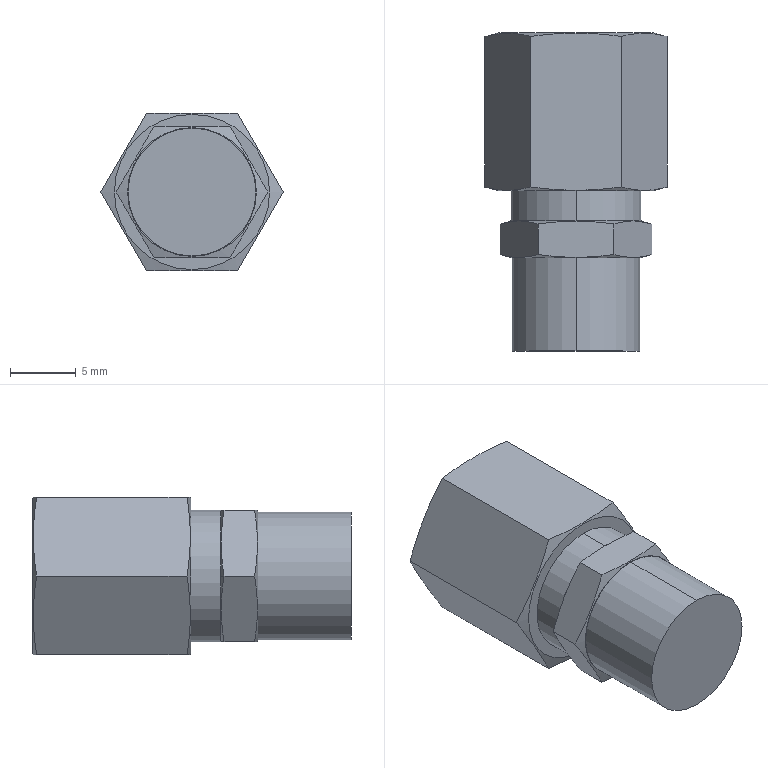Part | STEP file | H06-01S | 1 solid | 32 faces | box 13.856 x 24.2 x 12 mm | volume 1991 mm3 | plane 18 | cone 8 | cylinder 6 | commonest cylinder face diameters 6 x2 9.728 x2 10 x2
STEP:
#1=CARTESIAN_POINT('',(0.,5.1,-3.));
#2=VERTEX_POINT('',#1);
#3=CARTESIAN_POINT('',(0.,5.1,3.));
#4=VERTEX_POINT('',#3);
#5=CARTESIAN_POINT('',(0.,5.1,0.));
#6=DIRECTION('',(0.,1.,0.));
#7=DIRECTION('',(0.,0.,1.));
#8=AXIS2_PLACEMENT_3D('',#5,#6,#7);
#9=CIRCLE('',#8,3.);
#10=EDGE_CURVE('',#2,#4,#9,.T.);
#11=ORIENTED_EDGE('',*,*,#10,.F.);
#12=CARTESIAN_POINT('',(0.,21.1,-3.));
#13=VERTEX_POINT('',#12);
#14=CARTESIAN_POINT('',(0.,5.1,-3.));
#15=DIRECTION('',(0.,1.,0.));
#16=VECTOR('',#15,1000.);
#17=LINE('',#14,#16);
#18=EDGE_CURVE('',#2,#13,#17,.T.);
#19=ORIENTED_EDGE('',*,*,#18,.T.);
#20=CARTESIAN_POINT('',(0.,21.1,3.));
#21=VERTEX_POINT('',#20);
#22=CARTESIAN_POINT('',(0.,21.1,0.));
#23=DIRECTION('',(0.,-1.,0.));
#24=DIRECTION('',(0.,0.,1.));
#25=AXIS2_PLACEMENT_3D('',#22,#23,#24);
#26=CIRCLE('',#25,3.);
#27=EDGE_CURVE('',#21,#13,#26,.T.);
#28=ORIENTED_EDGE('',*,*,#27,.F.);
#29=CARTESIAN_POINT('',(0.,5.1,3.));
#30=DIRECTION('',(0.,1.,0.));
#31=VECTOR('',#30,1000.);
#32=LINE('',#29,#31);
#33=EDGE_CURVE('',#4,#21,#32,.T.);
#34=ORIENTED_EDGE('',*,*,#33,.F.);
#35=EDGE_LOOP('',(#11,#19,#28,#34));
#36=FACE_OUTER_BOUND('',#35,.T.);
#37=CARTESIAN_POINT('',(0.,5.1,0.));
#38=DIRECTION('',(0.,1.,0.));
#39=DIRECTION('',(0.,0.,1.));
#40=AXIS2_PLACEMENT_3D('',#37,#38,#39);
#41=CYLINDRICAL_SURFACE('',#40,3.);
#42=ADVANCED_FACE('',(#36),#41,.F.);
#43=CARTESIAN_POINT('',(0.,21.1,-5.9));
#44=VERTEX_POINT('',#43);
#45=CARTESIAN_POINT('',(0.,21.1,5.9));
#46=VERTEX_POINT('',#45);
#47=CARTESIAN_POINT('',(0.,21.1,0.));
#48=DIRECTION('',(0.,-1.,0.));
#49=DIRECTION('',(0.,0.,-1.));
#50=AXIS2_PLACEMENT_3D('',#47,#48,#49);
#51=CIRCLE('',#50,5.9);
#52=EDGE_CURVE('',#44,#46,#51,.T.);
#53=ORIENTED_EDGE('',*,*,#52,.T.);
#54=CARTESIAN_POINT('',(0.,21.073,6.));
#55=VERTEX_POINT('',#54);
#56=CARTESIAN_POINT('',(0.,20.823,6.934));
#57=DIRECTION('',(0.,-0.2588,0.9659));
#58=VECTOR('',#57,1000.);
#59=LINE('',#56,#58);
#60=EDGE_CURVE('',#46,#55,#59,.T.);
#61=ORIENTED_EDGE('',*,*,#60,.T.);
#62=CARTESIAN_POINT('',(3.464,20.824,6.));
#63=VERTEX_POINT('',#62);
#64=CARTESIAN_POINT('',(0.,21.073,6.));
#65=CARTESIAN_POINT('',(1.155,21.073,6.));
#66=CARTESIAN_POINT('',(2.309,20.979,6.));
#67=CARTESIAN_POINT('',(3.464,20.824,6.));
#68=B_SPLINE_CURVE_WITH_KNOTS('',3,(#64,#65,#66,#67),.UNSPECIFIED.,.F.,.F.,(4,4),(0.003464,0.006928),.UNSPECIFIED.);
#69=EDGE_CURVE('',#55,#63,#68,.T.);
#70=ORIENTED_EDGE('',*,*,#69,.T.);
#71=CARTESIAN_POINT('',(6.928,20.824,0.000000051));
#72=VERTEX_POINT('',#71);
#73=CARTESIAN_POINT('',(3.464,20.824,6.));
#74=CARTESIAN_POINT('',(4.041,20.979,5.));
#75=CARTESIAN_POINT('',(5.196,21.167,3.));
#76=CARTESIAN_POINT('',(6.351,20.979,1.));
#77=CARTESIAN_POINT('',(6.928,20.824,0.000000051));
#78=B_SPLINE_CURVE_WITH_KNOTS('',3,(#73,#74,#75,#76,#77),.UNSPECIFIED.,.F.,.F.,(4,1,4),(0.,0.003464,0.006928),.UNSPECIFIED.);
#79=EDGE_CURVE('',#63,#72,#78,.T.);
#80=ORIENTED_EDGE('',*,*,#79,.T.);
#81=CARTESIAN_POINT('',(3.464,20.824,-6.));
#82=VERTEX_POINT('',#81);
#83=CARTESIAN_POINT('',(6.928,20.824,0.000000051));
#84=CARTESIAN_POINT('',(6.351,20.979,-1.));
#85=CARTESIAN_POINT('',(5.196,21.167,-3.));
#86=CARTESIAN_POINT('',(4.041,20.979,-5.));
#87=CARTESIAN_POINT('',(3.464,20.824,-6.));
#88=B_SPLINE_CURVE_WITH_KNOTS('',3,(#83,#84,#85,#86,#87),.UNSPECIFIED.,.F.,.F.,(4,1,4),(0.,0.003464,0.006928),.UNSPECIFIED.);
#89=EDGE_CURVE('',#72,#82,#88,.T.);
#90=ORIENTED_EDGE('',*,*,#89,.T.);
#91=CARTESIAN_POINT('',(0.,21.073,-6.));
#92=VERTEX_POINT('',#91);
#93=CARTESIAN_POINT('',(3.464,20.824,-6.));
#94=CARTESIAN_POINT('',(2.309,20.979,-6.));
#95=CARTESIAN_POINT('',(1.155,21.073,-6.));
#96=CARTESIAN_POINT('',(0.,21.073,-6.));
#97=B_SPLINE_CURVE_WITH_KNOTS('',3,(#93,#94,#95,#96),.UNSPECIFIED.,.F.,.F.,(4,4),(0.,0.003464),.UNSPECIFIED.);
#98=EDGE_CURVE('',#82,#92,#97,.T.);
#99=ORIENTED_EDGE('',*,*,#98,.T.);
#100=CARTESIAN_POINT('',(0.,20.823,-6.934));
#101=DIRECTION('',(0.,-0.2588,-0.9659));
#102=VECTOR('',#101,1000.);
#103=LINE('',#100,#102);
#104=EDGE_CURVE('',#44,#92,#103,.T.);
#105=ORIENTED_EDGE('',*,*,#104,.F.);
#106=EDGE_LOOP('',(#53,#61,#70,#80,#90,#99,#105));
#107=FACE_OUTER_BOUND('',#106,.T.);
#108=CARTESIAN_POINT('',(0.,20.823,0.));
#109=DIRECTION('',(0.,-1.,0.));
#110=DIRECTION('',(0.,0.,-1.));
#111=AXIS2_PLACEMENT_3D('',#108,#109,#110);
#112=CONICAL_SURFACE('',#111,6.934,1.309);
#113=ADVANCED_FACE('',(#107),#112,.T.);
#114=CARTESIAN_POINT('',(0.,9.1,5.9));
#115=VERTEX_POINT('',#114);
#116=CARTESIAN_POINT('',(0.,9.1,-5.9));
#117=VERTEX_POINT('',#116);
#118=CARTESIAN_POINT('',(0.,9.1,0.));
#119=DIRECTION('',(0.,1.,0.));
#120=DIRECTION('',(0.,0.,1.));
#121=AXIS2_PLACEMENT_3D('',#118,#119,#120);
#122=CIRCLE('',#121,5.9);
#123=EDGE_CURVE('',#115,#117,#122,.T.);
#124=ORIENTED_EDGE('',*,*,#123,.T.);
#125=CARTESIAN_POINT('',(0.,9.127,-6.));
#126=VERTEX_POINT('',#125);
#127=CARTESIAN_POINT('',(0.,9.377,-6.934));
#128=DIRECTION('',(0.,0.2588,-0.9659));
#129=VECTOR('',#128,1000.);
#130=LINE('',#127,#129);
#131=EDGE_CURVE('',#117,#126,#130,.T.);
#132=ORIENTED_EDGE('',*,*,#131,.T.);
#133=CARTESIAN_POINT('',(3.464,9.376,-6.));
#134=VERTEX_POINT('',#133);
#135=CARTESIAN_POINT('',(3.464,9.376,-6.));
#136=CARTESIAN_POINT('',(2.309,9.221,-6.));
#137=CARTESIAN_POINT('',(1.155,9.127,-6.));
#138=CARTESIAN_POINT('',(0.,9.127,-6.));
#139=B_SPLINE_CURVE_WITH_KNOTS('',3,(#135,#136,#137,#138),.UNSPECIFIED.,.F.,.F.,(4,4),(0.,0.003464),.UNSPECIFIED.);
#140=EDGE_CURVE('',#134,#126,#139,.T.);
#141=ORIENTED_EDGE('',*,*,#140,.F.);
#142=CARTESIAN_POINT('',(6.928,9.376,0.));
#143=VERTEX_POINT('',#142);
#144=CARTESIAN_POINT('',(6.928,9.376,0.));
#145=CARTESIAN_POINT('',(6.351,9.221,-1.));
#146=CARTESIAN_POINT('',(5.196,9.033,-3.));
#147=CARTESIAN_POINT('',(4.041,9.221,-5.));
#148=CARTESIAN_POINT('',(3.464,9.376,-6.));
#149=B_SPLINE_CURVE_WITH_KNOTS('',3,(#144,#145,#146,#147,#148),.UNSPECIFIED.,.F.,.F.,(4,1,4),(0.,0.003464,0.006928),.UNSPECIFIED.);
#150=EDGE_CURVE('',#143,#134,#149,.T.);
#151=ORIENTED_EDGE('',*,*,#150,.F.);
#152=CARTESIAN_POINT('',(3.464,9.376,6.));
#153=VERTEX_POINT('',#152);
#154=CARTESIAN_POINT('',(3.464,9.376,6.));
#155=CARTESIAN_POINT('',(4.041,9.221,5.));
#156=CARTESIAN_POINT('',(5.196,9.033,3.));
#157=CARTESIAN_POINT('',(6.351,9.221,1.));
#158=CARTESIAN_POINT('',(6.928,9.376,0.));
#159=B_SPLINE_CURVE_WITH_KNOTS('',3,(#154,#155,#156,#157,#158),.UNSPECIFIED.,.F.,.F.,(4,1,4),(0.,0.003464,0.006928),.UNSPECIFIED.);
#160=EDGE_CURVE('',#153,#143,#159,.T.);
#161=ORIENTED_EDGE('',*,*,#160,.F.);
#162=CARTESIAN_POINT('',(0.,9.127,6.));
#163=VERTEX_POINT('',#162);
#164=CARTESIAN_POINT('',(0.,9.127,6.));
#165=CARTESIAN_POINT('',(1.155,9.127,6.));
#166=CARTESIAN_POINT('',(2.309,9.221,6.));
#167=CARTESIAN_POINT('',(3.464,9.376,6.));
#168=B_SPLINE_CURVE_WITH_KNOTS('',3,(#164,#165,#166,#167),.UNSPECIFIED.,.F.,.F.,(4,4),(0.003464,0.006928),.UNSPECIFIED.);
#169=EDGE_CURVE('',#163,#153,#168,.T.);
#170=ORIENTED_EDGE('',*,*,#169,.F.);
#171=CARTESIAN_POINT('',(0.,9.377,6.934));
#172=DIRECTION('',(0.,0.2588,0.9659));
#173=VECTOR('',#172,1000.);
#174=LINE('',#171,#173);
#175=EDGE_CURVE('',#115,#163,#174,.T.);
#176=ORIENTED_EDGE('',*,*,#175,.F.);
#177=EDGE_LOOP('',(#124,#132,#141,#151,#161,#170,#176));
#178=FACE_OUTER_BOUND('',#177,.T.);
#179=CARTESIAN_POINT('',(0.,9.377,0.));
#180=DIRECTION('',(0.,1.,0.));
#181=DIRECTION('',(0.,0.,1.));
#182=AXIS2_PLACEMENT_3D('',#179,#180,#181);
#183=CONICAL_SURFACE('',#182,6.934,1.309);
#184=ADVANCED_FACE('',(#178),#183,.T.);
#185=CARTESIAN_POINT('',(0.,9.1,-5.));
#186=VERTEX_POINT('',#185);
#187=CARTESIAN_POINT('',(0.,9.1,5.));
#188=VERTEX_POINT('',#187);
#189=CARTESIAN_POINT('',(0.,9.1,0.));
#190=DIRECTION('',(0.,-1.,0.));
#191=DIRECTION('',(0.,0.,-1.));
#192=AXIS2_PLACEMENT_3D('',#189,#190,#191);
#193=CIRCLE('',#192,5.);
#194=EDGE_CURVE('',#186,#188,#193,.T.);
#195=ORIENTED_EDGE('',*,*,#194,.T.);
#196=CARTESIAN_POINT('',(0.,6.8,5.));
#197=VERTEX_POINT('',#196);
#198=CARTESIAN_POINT('',(0.,21.1,5.));
#199=DIRECTION('',(0.,-1.,0.));
#200=VECTOR('',#199,1000.);
#201=LINE('',#198,#200);
#202=EDGE_CURVE('',#188,#197,#201,.T.);
#203=ORIENTED_EDGE('',*,*,#202,.T.);
#204=CARTESIAN_POINT('',(0.,6.8,-5.));
#205=VERTEX_POINT('',#204);
#206=CARTESIAN_POINT('',(0.,6.8,0.));
#207=DIRECTION('',(0.,1.,0.));
#208=DIRECTION('',(0.,0.,-1.));
#209=AXIS2_PLACEMENT_3D('',#206,#207,#208);
#210=CIRCLE('',#209,5.);
#211=EDGE_CURVE('',#197,#205,#210,.T.);
#212=ORIENTED_EDGE('',*,*,#211,.T.);
#213=CARTESIAN_POINT('',(0.,21.1,-5.));
#214=DIRECTION('',(0.,-1.,0.));
#215=VECTOR('',#214,1000.);
#216=LINE('',#213,#215);
#217=EDGE_CURVE('',#186,#205,#216,.T.);
#218=ORIENTED_EDGE('',*,*,#217,.F.);
#219=EDGE_LOOP('',(#195,#203,#212,#218));
#220=FACE_OUTER_BOUND('',#219,.T.);
#221=CARTESIAN_POINT('',(0.,21.1,0.));
#222=DIRECTION('',(0.,-1.,0.));
#223=DIRECTION('',(0.,0.,-1.));
#224=AXIS2_PLACEMENT_3D('',#221,#222,#223);
#225=CYLINDRICAL_SURFACE('',#224,5.);
#226=ADVANCED_FACE('',(#220),#225,.T.);
#227=CARTESIAN_POINT('',(4.9,6.8,0.));
#228=VERTEX_POINT('',#227);
#229=CARTESIAN_POINT('',(-4.9,6.8,0.));
#230=VERTEX_POINT('',#229);
#231=CARTESIAN_POINT('',(0.,6.8,0.));
#232=DIRECTION('',(0.,-1.,0.));
#233=DIRECTION('',(1.,0.,0.));
#234=AXIS2_PLACEMENT_3D('',#231,#232,#233);
#235=CIRCLE('',#234,4.9);
#236=EDGE_CURVE('',#228,#230,#235,.T.);
#237=ORIENTED_EDGE('',*,*,#236,.T.);
#238=CARTESIAN_POINT('',(-5.774,6.566,-0.000000051));
#239=VERTEX_POINT('',#238);
#240=CARTESIAN_POINT('',(-5.779,6.565,0.));
#241=DIRECTION('',(-0.9659,-0.2588,0.));
#242=VECTOR('',#241,1000.);
#243=LINE('',#240,#242);
#244=EDGE_CURVE('',#230,#239,#243,.T.);
#245=ORIENTED_EDGE('',*,*,#244,.T.);
#246=CARTESIAN_POINT('',(-2.887,6.566,5.));
#247=VERTEX_POINT('',#246);
#248=CARTESIAN_POINT('',(-5.774,6.566,-0.000000051));
#249=CARTESIAN_POINT('',(-5.292,6.695,0.8333));
#250=CARTESIAN_POINT('',(-4.33,6.852,2.5));
#251=CARTESIAN_POINT('',(-3.368,6.695,4.167));
#252=CARTESIAN_POINT('',(-2.887,6.566,5.));
#253=B_SPLINE_CURVE_WITH_KNOTS('',3,(#248,#249,#250,#251,#252),.UNSPECIFIED.,.F.,.F.,(4,1,4),(0.,0.002887,0.005774),.UNSPECIFIED.);
#254=EDGE_CURVE('',#239,#247,#253,.T.);
#255=ORIENTED_EDGE('',*,*,#254,.T.);
#256=CARTESIAN_POINT('',(2.887,6.566,5.));
#257=VERTEX_POINT('',#256);
#258=CARTESIAN_POINT('',(-2.887,6.566,5.));
#259=CARTESIAN_POINT('',(-1.925,6.695,5.));
#260=CARTESIAN_POINT('',(-0.000000077,6.852,5.));
#261=CARTESIAN_POINT('',(1.925,6.695,5.));
#262=CARTESIAN_POINT('',(2.887,6.566,5.));
#263=B_SPLINE_CURVE_WITH_KNOTS('',3,(#258,#259,#260,#261,#262),.UNSPECIFIED.,.F.,.F.,(4,1,4),(0.,0.002887,0.005774),.UNSPECIFIED.);
#264=EDGE_CURVE('',#247,#257,#263,.T.);
#265=ORIENTED_EDGE('',*,*,#264,.T.);
#266=CARTESIAN_POINT('',(5.774,6.566,0.000000006));
#267=VERTEX_POINT('',#266);
#268=CARTESIAN_POINT('',(2.887,6.566,5.));
#269=CARTESIAN_POINT('',(3.368,6.695,4.167));
#270=CARTESIAN_POINT('',(4.33,6.852,2.5));
#271=CARTESIAN_POINT('',(5.292,6.695,0.8333));
#272=CARTESIAN_POINT('',(5.774,6.566,0.000000006));
#273=B_SPLINE_CURVE_WITH_KNOTS('',3,(#268,#269,#270,#271,#272),.UNSPECIFIED.,.F.,.F.,(4,1,4),(0.,0.002887,0.005774),.UNSPECIFIED.);
#274=EDGE_CURVE('',#257,#267,#273,.T.);
#275=ORIENTED_EDGE('',*,*,#274,.T.);
#276=CARTESIAN_POINT('',(5.779,6.565,0.));
#277=DIRECTION('',(0.9659,-0.2588,0.));
#278=VECTOR('',#277,1000.);
#279=LINE('',#276,#278);
#280=EDGE_CURVE('',#228,#267,#279,.T.);
#281=ORIENTED_EDGE('',*,*,#280,.F.);
#282=EDGE_LOOP('',(#237,#245,#255,#265,#275,#281));
#283=FACE_OUTER_BOUND('',#282,.T.);
#284=CARTESIAN_POINT('',(0.,6.565,0.));
#285=DIRECTION('',(0.,-1.,0.));
#286=DIRECTION('',(1.,0.,0.));
#287=AXIS2_PLACEMENT_3D('',#284,#285,#286);
#288=CONICAL_SURFACE('',#287,5.779,1.309);
#289=ADVANCED_FACE('',(#283),#288,.T.);
#290=CARTESIAN_POINT('',(0.,4.,4.9));
#291=VERTEX_POINT('',#290);
#292=CARTESIAN_POINT('',(0.,4.,-4.9));
#293=VERTEX_POINT('',#292);
#294=CARTESIAN_POINT('',(0.,4.,0.));
#295=DIRECTION('',(0.,1.,0.));
#296=DIRECTION('',(0.,0.,1.));
#297=AXIS2_PLACEMENT_3D('',#294,#295,#296);
#298=CIRCLE('',#297,4.9);
#299=EDGE_CURVE('',#291,#293,#298,.T.);
#300=ORIENTED_EDGE('',*,*,#299,.T.);
#301=CARTESIAN_POINT('',(0.,4.027,-5.));
#302=VERTEX_POINT('',#301);
#303=CARTESIAN_POINT('',(0.,4.235,-5.779));
#304=DIRECTION('',(0.,0.2588,-0.9659));
#305=VECTOR('',#304,1000.);
#306=LINE('',#303,#305);
#307=EDGE_CURVE('',#293,#302,#306,.T.);
#308=ORIENTED_EDGE('',*,*,#307,.T.);
#309=CARTESIAN_POINT('',(2.887,4.234,-5.));
#310=VERTEX_POINT('',#309);
#311=CARTESIAN_POINT('',(2.887,4.234,-5.));
#312=CARTESIAN_POINT('',(1.925,4.105,-5.));
#313=CARTESIAN_POINT('',(0.9623,4.027,-5.));
#314=CARTESIAN_POINT('',(0.,4.027,-5.));
#315=B_SPLINE_CURVE_WITH_KNOTS('',3,(#311,#312,#313,#314),.UNSPECIFIED.,.F.,.F.,(4,4),(0.,0.002887),.UNSPECIFIED.);
#316=EDGE_CURVE('',#310,#302,#315,.T.);
#317=ORIENTED_EDGE('',*,*,#316,.F.);
#318=CARTESIAN_POINT('',(5.774,4.234,0.));
#319=VERTEX_POINT('',#318);
#320=CARTESIAN_POINT('',(5.774,4.234,0.));
#321=CARTESIAN_POINT('',(5.292,4.105,-0.8333));
#322=CARTESIAN_POINT('',(4.33,3.948,-2.5));
#323=CARTESIAN_POINT('',(3.368,4.105,-4.167));
#324=CARTESIAN_POINT('',(2.887,4.234,-5.));
#325=B_SPLINE_CURVE_WITH_KNOTS('',3,(#320,#321,#322,#323,#324),.UNSPECIFIED.,.F.,.F.,(4,1,4),(0.,0.002887,0.005774),.UNSPECIFIED.);
#326=EDGE_CURVE('',#319,#310,#325,.T.);
#327=ORIENTED_EDGE('',*,*,#326,.F.);
#328=CARTESIAN_POINT('',(2.887,4.234,5.));
#329=VERTEX_POINT('',#328);
#330=CARTESIAN_POINT('',(2.887,4.234,5.));
#331=CARTESIAN_POINT('',(3.368,4.105,4.167));
#332=CARTESIAN_POINT('',(4.33,3.948,2.5));
#333=CARTESIAN_POINT('',(5.292,4.105,0.8333));
#334=CARTESIAN_POINT('',(5.774,4.234,0.));
#335=B_SPLINE_CURVE_WITH_KNOTS('',3,(#330,#331,#332,#333,#334),.UNSPECIFIED.,.F.,.F.,(4,1,4),(0.,0.002887,0.005774),.UNSPECIFIED.);
#336=EDGE_CURVE('',#329,#319,#335,.T.);
#337=ORIENTED_EDGE('',*,*,#336,.F.);
#338=CARTESIAN_POINT('',(0.,4.027,5.));
#339=VERTEX_POINT('',#338);
#340=CARTESIAN_POINT('',(0.,4.027,5.));
#341=CARTESIAN_POINT('',(0.9623,4.027,5.));
#342=CARTESIAN_POINT('',(1.925,4.105,5.));
#343=CARTESIAN_POINT('',(2.887,4.234,5.));
#344=B_SPLINE_CURVE_WITH_KNOTS('',3,(#340,#341,#342,#343),.UNSPECIFIED.,.F.,.F.,(4,4),(0.002887,0.005774),.UNSPECIFIED.);
#345=EDGE_CURVE('',#339,#329,#344,.T.);
#346=ORIENTED_EDGE('',*,*,#345,.F.);
#347=CARTESIAN_POINT('',(0.,4.235,5.779));
#348=DIRECTION('',(0.,0.2588,0.9659));
#349=VECTOR('',#348,1000.);
#350=LINE('',#347,#349);
#351=EDGE_CURVE('',#291,#339,#350,.T.);
#352=ORIENTED_EDGE('',*,*,#351,.F.);
#353=EDGE_LOOP('',(#300,#308,#317,#327,#337,#346,#352));
#354=FACE_OUTER_BOUND('',#353,.T.);
#355=CARTESIAN_POINT('',(0.,4.235,0.));
#356=DIRECTION('',(0.,1.,0.));
#357=DIRECTION('',(0.,0.,1.));
#358=AXIS2_PLACEMENT_3D('',#355,#356,#357);
#359=CONICAL_SURFACE('',#358,5.779,1.309);
#360=ADVANCED_FACE('',(#354),#359,.T.);
#361=CARTESIAN_POINT('',(0.,4.,-4.864));
#362=VERTEX_POINT('',#361);
#363=CARTESIAN_POINT('',(0.,4.,4.864));
#364=VERTEX_POINT('',#363);
#365=CARTESIAN_POINT('',(0.,4.,0.));
#366=DIRECTION('',(0.,-1.,0.));
#367=DIRECTION('',(0.,0.,-1.));
#368=AXIS2_PLACEMENT_3D('',#365,#366,#367);
#369=CIRCLE('',#368,4.864);
#370=EDGE_CURVE('',#362,#364,#369,.T.);
#371=ORIENTED_EDGE('',*,*,#370,.T.);
#372=CARTESIAN_POINT('',(0.,-3.1,4.864));
#373=VERTEX_POINT('',#372);
#374=CARTESIAN_POINT('',(0.,21.1,4.864));
#375=DIRECTION('',(0.,-1.,0.));
#376=VECTOR('',#375,1000.);
#377=LINE('',#374,#376);
#378=EDGE_CURVE('',#364,#373,#377,.T.);
#379=ORIENTED_EDGE('',*,*,#378,.T.);
#380=CARTESIAN_POINT('',(0.,-3.1,-4.864));
#381=VERTEX_POINT('',#380);
#382=CARTESIAN_POINT('',(0.,-3.1,0.));
#383=DIRECTION('',(0.,1.,0.));
#384=DIRECTION('',(0.,0.,-1.));
#385=AXIS2_PLACEMENT_3D('',#382,#383,#384);
#386=CIRCLE('',#385,4.864);
#387=EDGE_CURVE('',#373,#381,#386,.T.);
#388=ORIENTED_EDGE('',*,*,#387,.T.);
#389=CARTESIAN_POINT('',(0.,21.1,-4.864));
#390=DIRECTION('',(0.,-1.,0.));
#391=VECTOR('',#390,1000.);
#392=LINE('',#389,#391);
#393=EDGE_CURVE('',#362,#381,#392,.T.);
#394=ORIENTED_EDGE('',*,*,#393,.F.);
#395=EDGE_LOOP('',(#371,#379,#388,#394));
#396=FACE_OUTER_BOUND('',#395,.T.);
#397=CARTESIAN_POINT('',(0.,21.1,0.));
#398=DIRECTION('',(0.,-1.,0.));
#399=DIRECTION('',(0.,0.,-1.));
#400=AXIS2_PLACEMENT_3D('',#397,#398,#399);
#401=CYLINDRICAL_SURFACE('',#400,4.864);
#402=ADVANCED_FACE('',(#396),#401,.T.);
#403=ORIENTED_EDGE('',*,*,#18,.F.);
#404=CARTESIAN_POINT('',(0.,5.1,0.));
#405=DIRECTION('',(0.,1.,0.));
#406=DIRECTION('',(0.,0.,1.));
#407=AXIS2_PLACEMENT_3D('',#404,#405,#406);
#408=CIRCLE('',#407,3.);
#409=EDGE_CURVE('',#4,#2,#408,.T.);
#410=ORIENTED_EDGE('',*,*,#409,.F.);
#411=ORIENTED_EDGE('',*,*,#33,.T.);
#412=CARTESIAN_POINT('',(0.,21.1,0.));
#413=DIRECTION('',(0.,-1.,0.));
#414=DIRECTION('',(0.,0.,1.));
#415=AXIS2_PLACEMENT_3D('',#412,#413,#414);
#416=CIRCLE('',#415,3.);
#417=EDGE_CURVE('',#13,#21,#416,.T.);
#418=ORIENTED_EDGE('',*,*,#417,.F.);
#419=EDGE_LOOP('',(#403,#410,#411,#418));
#420=FACE_OUTER_BOUND('',#419,.T.);
#421=CARTESIAN_POINT('',(0.,5.1,0.));
#422=DIRECTION('',(0.,1.,0.));
#423=DIRECTION('',(0.,0.,1.));
#424=AXIS2_PLACEMENT_3D('',#421,#422,#423);
#425=CYLINDRICAL_SURFACE('',#424,3.);
#426=ADVANCED_FACE('',(#420),#425,.F.);
#427=ORIENTED_EDGE('',*,*,#52,.F.);
#428=CARTESIAN_POINT('',(0.,21.1,0.));
#429=DIRECTION('',(0.,-1.,0.));
#430=DIRECTION('',(0.,0.,-1.));
#431=AXIS2_PLACEMENT_3D('',#428,#429,#430);
#432=CIRCLE('',#431,5.9);
#433=EDGE_CURVE('',#46,#44,#432,.T.);
#434=ORIENTED_EDGE('',*,*,#433,.F.);
#435=EDGE_LOOP('',(#427,#434));
#436=FACE_OUTER_BOUND('',#435,.T.);
#437=ORIENTED_EDGE('',*,*,#27,.T.);
#438=ORIENTED_EDGE('',*,*,#417,.T.);
#439=EDGE_LOOP('',(#437,#438));
#440=FACE_BOUND('',#439,.T.);
#441=CARTESIAN_POINT('',(-5.9,21.1,0.));
#442=DIRECTION('',(0.,-1.,0.));
#443=DIRECTION('',(0.,0.,-1.));
#444=AXIS2_PLACEMENT_3D('',#441,#442,#443);
#445=PLANE('',#444);
#446=ADVANCED_FACE('',(#436,#440),#445,.F.);
#447=ORIENTED_EDGE('',*,*,#409,.T.);
#448=ORIENTED_EDGE('',*,*,#10,.T.);
#449=EDGE_LOOP('',(#447,#448));
#450=FACE_OUTER_BOUND('',#449,.T.);
#451=CARTESIAN_POINT('',(3.,5.1,0.));
#452=DIRECTION('',(0.,1.,0.));
#453=DIRECTION('',(0.,0.,1.));
#454=AXIS2_PLACEMENT_3D('',#451,#452,#453);
#455=PLANE('',#454);
#456=ADVANCED_FACE('',(#450),#455,.T.);
#457=ORIENTED_EDGE('',*,*,#60,.F.);
#458=ORIENTED_EDGE('',*,*,#433,.T.);
#459=ORIENTED_EDGE('',*,*,#104,.T.);
#460=CARTESIAN_POINT('',(-3.464,20.824,-6.));
#461=VERTEX_POINT('',#460);
#462=CARTESIAN_POINT('',(0.,21.073,-6.));
#463=CARTESIAN_POINT('',(-1.155,21.073,-6.));
#464=CARTESIAN_POINT('',(-2.309,20.979,-6.));
#465=CARTESIAN_POINT('',(-3.464,20.824,-6.));
#466=B_SPLINE_CURVE_WITH_KNOTS('',3,(#462,#463,#464,#465),.UNSPECIFIED.,.F.,.F.,(4,4),(0.003464,0.006928),.UNSPECIFIED.);
#467=EDGE_CURVE('',#92,#461,#466,.T.);
#468=ORIENTED_EDGE('',*,*,#467,.T.);
#469=CARTESIAN_POINT('',(-6.928,20.824,-0.000000051));
#470=VERTEX_POINT('',#469);
#471=CARTESIAN_POINT('',(-3.464,20.824,-6.));
#472=CARTESIAN_POINT('',(-4.041,20.979,-5.));
#473=CARTESIAN_POINT('',(-5.196,21.167,-3.));
#474=CARTESIAN_POINT('',(-6.351,20.979,-1.));
#475=CARTESIAN_POINT('',(-6.928,20.824,-0.000000051));
#476=B_SPLINE_CURVE_WITH_KNOTS('',3,(#471,#472,#473,#474,#475),.UNSPECIFIED.,.F.,.F.,(4,1,4),(0.,0.003464,0.006928),.UNSPECIFIED.);
#477=EDGE_CURVE('',#461,#470,#476,.T.);
#478=ORIENTED_EDGE('',*,*,#477,.T.);
#479=CARTESIAN_POINT('',(-3.464,20.824,6.));
#480=VERTEX_POINT('',#479);
#481=CARTESIAN_POINT('',(-6.928,20.824,-0.000000051));
#482=CARTESIAN_POINT('',(-6.351,20.979,1.));
#483=CARTESIAN_POINT('',(-5.196,21.167,3.));
#484=CARTESIAN_POINT('',(-4.041,20.979,5.));
#485=CARTESIAN_POINT('',(-3.464,20.824,6.));
#486=B_SPLINE_CURVE_WITH_KNOTS('',3,(#481,#482,#483,#484,#485),.UNSPECIFIED.,.F.,.F.,(4,1,4),(0.,0.003464,0.006928),.UNSPECIFIED.);
#487=EDGE_CURVE('',#470,#480,#486,.T.);
#488=ORIENTED_EDGE('',*,*,#487,.T.);
#489=CARTESIAN_POINT('',(-3.464,20.824,6.));
#490=CARTESIAN_POINT('',(-2.309,20.979,6.));
#491=CARTESIAN_POINT('',(-1.155,21.073,6.));
#492=CARTESIAN_POINT('',(0.,21.073,6.));
#493=B_SPLINE_CURVE_WITH_KNOTS('',3,(#489,#490,#491,#492),.UNSPECIFIED.,.F.,.F.,(4,4),(0.,0.003464),.UNSPECIFIED.);
#494=EDGE_CURVE('',#480,#55,#493,.T.);
#495=ORIENTED_EDGE('',*,*,#494,.T.);
#496=EDGE_LOOP('',(#457,#458,#459,#468,#478,#488,#495));
#497=FACE_OUTER_BOUND('',#496,.T.);
#498=CARTESIAN_POINT('',(0.,20.823,0.));
#499=DIRECTION('',(0.,-1.,0.));
#500=DIRECTION('',(0.,0.,-1.));
#501=AXIS2_PLACEMENT_3D('',#498,#499,#500);
#502=CONICAL_SURFACE('',#501,6.934,1.309);
#503=ADVANCED_FACE('',(#497),#502,.T.);
#504=ORIENTED_EDGE('',*,*,#98,.F.);
#505=CARTESIAN_POINT('',(3.464,9.1,-6.));
#506=DIRECTION('',(0.,-1.,0.));
#507=VECTOR('',#506,1000.);
#508=LINE('',#505,#507);
#509=EDGE_CURVE('',#82,#134,#508,.T.);
#510=ORIENTED_EDGE('',*,*,#509,.T.);
#511=ORIENTED_EDGE('',*,*,#140,.T.);
#512=CARTESIAN_POINT('',(-3.464,9.376,-6.));
#513=VERTEX_POINT('',#512);
#514=CARTESIAN_POINT('',(0.,9.127,-6.));
#515=CARTESIAN_POINT('',(-1.155,9.127,-6.));
#516=CARTESIAN_POINT('',(-2.309,9.221,-6.));
#517=CARTESIAN_POINT('',(-3.464,9.376,-6.));
#518=B_SPLINE_CURVE_WITH_KNOTS('',3,(#514,#515,#516,#517),.UNSPECIFIED.,.F.,.F.,(4,4),(0.003464,0.006928),.UNSPECIFIED.);
#519=EDGE_CURVE('',#126,#513,#518,.T.);
#520=ORIENTED_EDGE('',*,*,#519,.T.);
#521=CARTESIAN_POINT('',(-3.464,9.1,-6.));
#522=DIRECTION('',(0.,1.,0.));
#523=VECTOR('',#522,1000.);
#524=LINE('',#521,#523);
#525=EDGE_CURVE('',#513,#461,#524,.T.);
#526=ORIENTED_EDGE('',*,*,#525,.T.);
#527=ORIENTED_EDGE('',*,*,#467,.F.);
#528=EDGE_LOOP('',(#504,#510,#511,#520,#526,#527));
#529=FACE_OUTER_BOUND('',#528,.T.);
#530=CARTESIAN_POINT('',(3.464,9.1,-6.));
#531=DIRECTION('',(0.,0.,-1.));
#532=DIRECTION('',(-1.,0.,0.));
#533=AXIS2_PLACEMENT_3D('',#530,#531,#532);
#534=PLANE('',#533);
#535=ADVANCED_FACE('',(#529),#534,.T.);
#536=ORIENTED_EDGE('',*,*,#89,.F.);
#537=CARTESIAN_POINT('',(6.928,9.1,0.));
#538=DIRECTION('',(0.,-1.,0.));
#539=VECTOR('',#538,1000.);
#540=LINE('',#537,#539);
#541=EDGE_CURVE('',#72,#143,#540,.T.);
#542=ORIENTED_EDGE('',*,*,#541,.T.);
#543=ORIENTED_EDGE('',*,*,#150,.T.);
#544=ORIENTED_EDGE('',*,*,#509,.F.);
#545=EDGE_LOOP('',(#536,#542,#543,#544));
#546=FACE_OUTER_BOUND('',#545,.T.);
#547=CARTESIAN_POINT('',(6.928,9.1,0.));
#548=DIRECTION('',(0.866,0.,-0.5));
#549=DIRECTION('',(-0.5,0.,-0.866));
#550=AXIS2_PLACEMENT_3D('',#547,#548,#549);
#551=PLANE('',#550);
#552=ADVANCED_FACE('',(#546),#551,.T.);
#553=ORIENTED_EDGE('',*,*,#79,.F.);
#554=CARTESIAN_POINT('',(3.464,9.1,6.));
#555=DIRECTION('',(0.,-1.,0.));
#556=VECTOR('',#555,1000.);
#557=LINE('',#554,#556);
#558=EDGE_CURVE('',#63,#153,#557,.T.);
#559=ORIENTED_EDGE('',*,*,#558,.T.);
#560=ORIENTED_EDGE('',*,*,#160,.T.);
#561=ORIENTED_EDGE('',*,*,#541,.F.);
#562=EDGE_LOOP('',(#553,#559,#560,#561));
#563=FACE_OUTER_BOUND('',#562,.T.);
#564=CARTESIAN_POINT('',(3.464,9.1,6.));
#565=DIRECTION('',(0.866,0.,0.5));
#566=DIRECTION('',(0.5,0.,-0.866));
#567=AXIS2_PLACEMENT_3D('',#564,#565,#566);
#568=PLANE('',#567);
#569=ADVANCED_FACE('',(#563),#568,.T.);
#570=ORIENTED_EDGE('',*,*,#494,.F.);
#571=CARTESIAN_POINT('',(-3.464,9.376,6.));
#572=VERTEX_POINT('',#571);
#573=CARTESIAN_POINT('',(-3.464,9.1,6.));
#574=DIRECTION('',(0.,-1.,0.));
#575=VECTOR('',#574,1000.);
#576=LINE('',#573,#575);
#577=EDGE_CURVE('',#480,#572,#576,.T.);
#578=ORIENTED_EDGE('',*,*,#577,.T.);
#579=CARTESIAN_POINT('',(-3.464,9.376,6.));
#580=CARTESIAN_POINT('',(-2.309,9.221,6.));
#581=CARTESIAN_POINT('',(-1.155,9.127,6.));
#582=CARTESIAN_POINT('',(0.,9.127,6.));
#583=B_SPLINE_CURVE_WITH_KNOTS('',3,(#579,#580,#581,#582),.UNSPECIFIED.,.F.,.F.,(4,4),(0.,0.003464),.UNSPECIFIED.);
#584=EDGE_CURVE('',#572,#163,#583,.T.);
#585=ORIENTED_EDGE('',*,*,#584,.T.);
#586=ORIENTED_EDGE('',*,*,#169,.T.);
#587=ORIENTED_EDGE('',*,*,#558,.F.);
#588=ORIENTED_EDGE('',*,*,#69,.F.);
#589=EDGE_LOOP('',(#570,#578,#585,#586,#587,#588));
#590=FACE_OUTER_BOUND('',#589,.T.);
#591=CARTESIAN_POINT('',(-3.464,9.1,6.));
#592=DIRECTION('',(0.,0.,1.));
#593=DIRECTION('',(1.,0.,0.));
#594=AXIS2_PLACEMENT_3D('',#591,#592,#593);
#595=PLANE('',#594);
#596=ADVANCED_FACE('',(#590),#595,.T.);
#597=ORIENTED_EDGE('',*,*,#487,.F.);
#598=CARTESIAN_POINT('',(-6.928,9.376,0.));
#599=VERTEX_POINT('',#598);
#600=CARTESIAN_POINT('',(-6.928,9.1,0.));
#601=DIRECTION('',(0.,-1.,0.));
#602=VECTOR('',#601,1000.);
#603=LINE('',#600,#602);
#604=EDGE_CURVE('',#470,#599,#603,.T.);
#605=ORIENTED_EDGE('',*,*,#604,.T.);
#606=CARTESIAN_POINT('',(-6.928,9.376,0.));
#607=CARTESIAN_POINT('',(-6.351,9.221,1.));
#608=CARTESIAN_POINT('',(-5.196,9.033,3.));
#609=CARTESIAN_POINT('',(-4.041,9.221,5.));
#610=CARTESIAN_POINT('',(-3.464,9.376,6.));
#611=B_SPLINE_CURVE_WITH_KNOTS('',3,(#606,#607,#608,#609,#610),.UNSPECIFIED.,.F.,.F.,(4,1,4),(0.,0.003464,0.006928),.UNSPECIFIED.);
#612=EDGE_CURVE('',#599,#572,#611,.T.);
#613=ORIENTED_EDGE('',*,*,#612,.T.);
#614=ORIENTED_EDGE('',*,*,#577,.F.);
#615=EDGE_LOOP('',(#597,#605,#613,#614));
#616=FACE_OUTER_BOUND('',#615,.T.);
#617=CARTESIAN_POINT('',(-6.928,9.1,0.));
#618=DIRECTION('',(-0.866,0.,0.5));
#619=DIRECTION('',(0.5,0.,0.866));
#620=AXIS2_PLACEMENT_3D('',#617,#618,#619);
#621=PLANE('',#620);
#622=ADVANCED_FACE('',(#616),#621,.T.);
#623=ORIENTED_EDGE('',*,*,#477,.F.);
#624=ORIENTED_EDGE('',*,*,#525,.F.);
#625=CARTESIAN_POINT('',(-3.464,9.376,-6.));
#626=CARTESIAN_POINT('',(-4.041,9.221,-5.));
#627=CARTESIAN_POINT('',(-5.196,9.033,-3.));
#628=CARTESIAN_POINT('',(-6.351,9.221,-1.));
#629=CARTESIAN_POINT('',(-6.928,9.376,0.));
#630=B_SPLINE_CURVE_WITH_KNOTS('',3,(#625,#626,#627,#628,#629),.UNSPECIFIED.,.F.,.F.,(4,1,4),(0.,0.003464,0.006928),.UNSPECIFIED.);
#631=EDGE_CURVE('',#513,#599,#630,.T.);
#632=ORIENTED_EDGE('',*,*,#631,.T.);
#633=ORIENTED_EDGE('',*,*,#604,.F.);
#634=EDGE_LOOP('',(#623,#624,#632,#633));
#635=FACE_OUTER_BOUND('',#634,.T.);
#636=CARTESIAN_POINT('',(-3.464,9.1,-6.));
#637=DIRECTION('',(-0.866,0.,-0.5));
#638=DIRECTION('',(-0.5,0.,0.866));
#639=AXIS2_PLACEMENT_3D('',#636,#637,#638);
#640=PLANE('',#639);
#641=ADVANCED_FACE('',(#635),#640,.T.);
#642=ORIENTED_EDGE('',*,*,#131,.F.);
#643=CARTESIAN_POINT('',(0.,9.1,0.));
#644=DIRECTION('',(0.,1.,0.));
#645=DIRECTION('',(0.,0.,1.));
#646=AXIS2_PLACEMENT_3D('',#643,#644,#645);
#647=CIRCLE('',#646,5.9);
#648=EDGE_CURVE('',#117,#115,#647,.T.);
#649=ORIENTED_EDGE('',*,*,#648,.T.);
#650=ORIENTED_EDGE('',*,*,#175,.T.);
#651=ORIENTED_EDGE('',*,*,#584,.F.);
#652=ORIENTED_EDGE('',*,*,#612,.F.);
#653=ORIENTED_EDGE('',*,*,#631,.F.);
#654=ORIENTED_EDGE('',*,*,#519,.F.);
#655=EDGE_LOOP('',(#642,#649,#650,#651,#652,#653,#654));
#656=FACE_OUTER_BOUND('',#655,.T.);
#657=CARTESIAN_POINT('',(0.,9.377,0.));
#658=DIRECTION('',(0.,1.,0.));
#659=DIRECTION('',(0.,0.,1.));
#660=AXIS2_PLACEMENT_3D('',#657,#658,#659);
#661=CONICAL_SURFACE('',#660,6.934,1.309);
#662=ADVANCED_FACE('',(#656),#661,.T.);
#663=ORIENTED_EDGE('',*,*,#194,.F.);
#664=CARTESIAN_POINT('',(0.,9.1,0.));
#665=DIRECTION('',(0.,-1.,0.));
#666=DIRECTION('',(0.,0.,-1.));
#667=AXIS2_PLACEMENT_3D('',#664,#665,#666);
#668=CIRCLE('',#667,5.);
#669=EDGE_CURVE('',#188,#186,#668,.T.);
#670=ORIENTED_EDGE('',*,*,#669,.F.);
#671=EDGE_LOOP('',(#663,#670));
#672=FACE_BOUND('',#671,.T.);
#673=ORIENTED_EDGE('',*,*,#123,.F.);
#674=ORIENTED_EDGE('',*,*,#648,.F.);
#675=EDGE_LOOP('',(#673,#674));
#676=FACE_OUTER_BOUND('',#675,.T.);
#677=CARTESIAN_POINT('',(-5.,9.1,0.));
#678=DIRECTION('',(0.,1.,0.));
#679=DIRECTION('',(0.,0.,1.));
#680=AXIS2_PLACEMENT_3D('',#677,#678,#679);
#681=PLANE('',#680);
#682=ADVANCED_FACE('',(#672,#676),#681,.F.);
#683=ORIENTED_EDGE('',*,*,#202,.F.);
#684=ORIENTED_EDGE('',*,*,#669,.T.);
#685=ORIENTED_EDGE('',*,*,#217,.T.);
#686=CARTESIAN_POINT('',(0.,6.8,0.));
#687=DIRECTION('',(0.,1.,0.));
#688=DIRECTION('',(0.,0.,-1.));
#689=AXIS2_PLACEMENT_3D('',#686,#687,#688);
#690=CIRCLE('',#689,5.);
#691=EDGE_CURVE('',#205,#197,#690,.T.);
#692=ORIENTED_EDGE('',*,*,#691,.T.);
#693=EDGE_LOOP('',(#683,#684,#685,#692));
#694=FACE_OUTER_BOUND('',#693,.T.);
#695=CARTESIAN_POINT('',(0.,21.1,0.));
#696=DIRECTION('',(0.,-1.,0.));
#697=DIRECTION('',(0.,0.,-1.));
#698=AXIS2_PLACEMENT_3D('',#695,#696,#697);
#699=CYLINDRICAL_SURFACE('',#698,5.);
#700=ADVANCED_FACE('',(#694),#699,.T.);
#701=ORIENTED_EDGE('',*,*,#236,.F.);
#702=CARTESIAN_POINT('',(0.,6.8,0.));
#703=DIRECTION('',(0.,-1.,0.));
#704=DIRECTION('',(1.,0.,0.));
#705=AXIS2_PLACEMENT_3D('',#702,#703,#704);
#706=CIRCLE('',#705,4.9);
#707=EDGE_CURVE('',#230,#228,#706,.T.);
#708=ORIENTED_EDGE('',*,*,#707,.F.);
#709=EDGE_LOOP('',(#701,#708));
#710=FACE_BOUND('',#709,.T.);
#711=ORIENTED_EDGE('',*,*,#691,.F.);
#712=ORIENTED_EDGE('',*,*,#211,.F.);
#713=EDGE_LOOP('',(#711,#712));
#714=FACE_OUTER_BOUND('',#713,.T.);
#715=CARTESIAN_POINT('',(-4.9,6.8,0.));
#716=DIRECTION('',(0.,1.,0.));
#717=DIRECTION('',(0.,0.,1.));
#718=AXIS2_PLACEMENT_3D('',#715,#716,#717);
#719=PLANE('',#718);
#720=ADVANCED_FACE('',(#710,#714),#719,.F.);
#721=ORIENTED_EDGE('',*,*,#244,.F.);
#722=ORIENTED_EDGE('',*,*,#707,.T.);
#723=ORIENTED_EDGE('',*,*,#280,.T.);
#724=CARTESIAN_POINT('',(2.887,6.566,-5.));
#725=VERTEX_POINT('',#724);
#726=CARTESIAN_POINT('',(5.774,6.566,0.000000006));
#727=CARTESIAN_POINT('',(5.292,6.695,-0.8333));
#728=CARTESIAN_POINT('',(4.33,6.852,-2.5));
#729=CARTESIAN_POINT('',(3.368,6.695,-4.167));
#730=CARTESIAN_POINT('',(2.887,6.566,-5.));
#731=B_SPLINE_CURVE_WITH_KNOTS('',3,(#726,#727,#728,#729,#730),.UNSPECIFIED.,.F.,.F.,(4,1,4),(0.,0.002887,0.005774),.UNSPECIFIED.);
#732=EDGE_CURVE('',#267,#725,#731,.T.);
#733=ORIENTED_EDGE('',*,*,#732,.T.);
#734=CARTESIAN_POINT('',(-2.887,6.566,-5.));
#735=VERTEX_POINT('',#734);
#736=CARTESIAN_POINT('',(2.887,6.566,-5.));
#737=CARTESIAN_POINT('',(1.925,6.695,-5.));
#738=CARTESIAN_POINT('',(0.00000003,6.852,-5.));
#739=CARTESIAN_POINT('',(-1.925,6.695,-5.));
#740=CARTESIAN_POINT('',(-2.887,6.566,-5.));
#741=B_SPLINE_CURVE_WITH_KNOTS('',3,(#736,#737,#738,#739,#740),.UNSPECIFIED.,.F.,.F.,(4,1,4),(0.,0.002887,0.005774),.UNSPECIFIED.);
#742=EDGE_CURVE('',#725,#735,#741,.T.);
#743=ORIENTED_EDGE('',*,*,#742,.T.);
#744=CARTESIAN_POINT('',(-2.887,6.566,-5.));
#745=CARTESIAN_POINT('',(-3.368,6.695,-4.167));
#746=CARTESIAN_POINT('',(-4.33,6.852,-2.5));
#747=CARTESIAN_POINT('',(-5.292,6.695,-0.8333));
#748=CARTESIAN_POINT('',(-5.774,6.566,-0.000000051));
#749=B_SPLINE_CURVE_WITH_KNOTS('',3,(#744,#745,#746,#747,#748),.UNSPECIFIED.,.F.,.F.,(4,1,4),(0.,0.002887,0.005774),.UNSPECIFIED.);
#750=EDGE_CURVE('',#735,#239,#749,.T.);
#751=ORIENTED_EDGE('',*,*,#750,.T.);
#752=EDGE_LOOP('',(#721,#722,#723,#733,#743,#751));
#753=FACE_OUTER_BOUND('',#752,.T.);
#754=CARTESIAN_POINT('',(0.,6.565,0.));
#755=DIRECTION('',(0.,-1.,0.));
#756=DIRECTION('',(1.,0.,0.));
#757=AXIS2_PLACEMENT_3D('',#754,#755,#756);
#758=CONICAL_SURFACE('',#757,5.779,1.309);
#759=ADVANCED_FACE('',(#753),#758,.T.);
#760=ORIENTED_EDGE('',*,*,#742,.F.);
#761=CARTESIAN_POINT('',(2.887,4.,-5.));
#762=DIRECTION('',(0.,-1.,0.));
#763=VECTOR('',#762,1000.);
#764=LINE('',#761,#763);
#765=EDGE_CURVE('',#725,#310,#764,.T.);
#766=ORIENTED_EDGE('',*,*,#765,.T.);
#767=ORIENTED_EDGE('',*,*,#316,.T.);
#768=CARTESIAN_POINT('',(-2.887,4.234,-5.));
#769=VERTEX_POINT('',#768);
#770=CARTESIAN_POINT('',(0.,4.027,-5.));
#771=CARTESIAN_POINT('',(-0.9623,4.027,-5.));
#772=CARTESIAN_POINT('',(-1.925,4.105,-5.));
#773=CARTESIAN_POINT('',(-2.887,4.234,-5.));
#774=B_SPLINE_CURVE_WITH_KNOTS('',3,(#770,#771,#772,#773),.UNSPECIFIED.,.F.,.F.,(4,4),(0.002887,0.005774),.UNSPECIFIED.);
#775=EDGE_CURVE('',#302,#769,#774,.T.);
#776=ORIENTED_EDGE('',*,*,#775,.T.);
#777=CARTESIAN_POINT('',(-2.887,4.,-5.));
#778=DIRECTION('',(0.,1.,0.));
#779=VECTOR('',#778,1000.);
#780=LINE('',#777,#779);
#781=EDGE_CURVE('',#769,#735,#780,.T.);
#782=ORIENTED_EDGE('',*,*,#781,.T.);
#783=EDGE_LOOP('',(#760,#766,#767,#776,#782));
#784=FACE_OUTER_BOUND('',#783,.T.);
#785=CARTESIAN_POINT('',(2.887,4.,-5.));
#786=DIRECTION('',(0.,0.,-1.));
#787=DIRECTION('',(-1.,0.,0.));
#788=AXIS2_PLACEMENT_3D('',#785,#786,#787);
#789=PLANE('',#788);
#790=ADVANCED_FACE('',(#784),#789,.T.);
#791=ORIENTED_EDGE('',*,*,#732,.F.);
#792=CARTESIAN_POINT('',(5.774,4.,0.));
#793=DIRECTION('',(0.,-1.,0.));
#794=VECTOR('',#793,1000.);
#795=LINE('',#792,#794);
#796=EDGE_CURVE('',#267,#319,#795,.T.);
#797=ORIENTED_EDGE('',*,*,#796,.T.);
#798=ORIENTED_EDGE('',*,*,#326,.T.);
#799=ORIENTED_EDGE('',*,*,#765,.F.);
#800=EDGE_LOOP('',(#791,#797,#798,#799));
#801=FACE_OUTER_BOUND('',#800,.T.);
#802=CARTESIAN_POINT('',(5.774,4.,0.));
#803=DIRECTION('',(0.866,0.,-0.5));
#804=DIRECTION('',(-0.5,0.,-0.866));
#805=AXIS2_PLACEMENT_3D('',#802,#803,#804);
#806=PLANE('',#805);
#807=ADVANCED_FACE('',(#801),#806,.T.);
#808=ORIENTED_EDGE('',*,*,#274,.F.);
#809=CARTESIAN_POINT('',(2.887,4.,5.));
#810=DIRECTION('',(0.,-1.,0.));
#811=VECTOR('',#810,1000.);
#812=LINE('',#809,#811);
#813=EDGE_CURVE('',#257,#329,#812,.T.);
#814=ORIENTED_EDGE('',*,*,#813,.T.);
#815=ORIENTED_EDGE('',*,*,#336,.T.);
#816=ORIENTED_EDGE('',*,*,#796,.F.);
#817=EDGE_LOOP('',(#808,#814,#815,#816));
#818=FACE_OUTER_BOUND('',#817,.T.);
#819=CARTESIAN_POINT('',(2.887,4.,5.));
#820=DIRECTION('',(0.866,0.,0.5));
#821=DIRECTION('',(0.5,0.,-0.866));
#822=AXIS2_PLACEMENT_3D('',#819,#820,#821);
#823=PLANE('',#822);
#824=ADVANCED_FACE('',(#818),#823,.T.);
#825=ORIENTED_EDGE('',*,*,#264,.F.);
#826=CARTESIAN_POINT('',(-2.887,4.234,5.));
#827=VERTEX_POINT('',#826);
#828=CARTESIAN_POINT('',(-2.887,4.,5.));
#829=DIRECTION('',(0.,-1.,0.));
#830=VECTOR('',#829,1000.);
#831=LINE('',#828,#830);
#832=EDGE_CURVE('',#247,#827,#831,.T.);
#833=ORIENTED_EDGE('',*,*,#832,.T.);
#834=CARTESIAN_POINT('',(-2.887,4.234,5.));
#835=CARTESIAN_POINT('',(-1.925,4.105,5.));
#836=CARTESIAN_POINT('',(-0.9623,4.027,5.));
#837=CARTESIAN_POINT('',(0.,4.027,5.));
#838=B_SPLINE_CURVE_WITH_KNOTS('',3,(#834,#835,#836,#837),.UNSPECIFIED.,.F.,.F.,(4,4),(0.,0.002887),.UNSPECIFIED.);
#839=EDGE_CURVE('',#827,#339,#838,.T.);
#840=ORIENTED_EDGE('',*,*,#839,.T.);
#841=ORIENTED_EDGE('',*,*,#345,.T.);
#842=ORIENTED_EDGE('',*,*,#813,.F.);
#843=EDGE_LOOP('',(#825,#833,#840,#841,#842));
#844=FACE_OUTER_BOUND('',#843,.T.);
#845=CARTESIAN_POINT('',(-2.887,4.,5.));
#846=DIRECTION('',(0.,0.,1.));
#847=DIRECTION('',(1.,0.,0.));
#848=AXIS2_PLACEMENT_3D('',#845,#846,#847);
#849=PLANE('',#848);
#850=ADVANCED_FACE('',(#844),#849,.T.);
#851=ORIENTED_EDGE('',*,*,#254,.F.);
#852=CARTESIAN_POINT('',(-5.774,4.234,0.));
#853=VERTEX_POINT('',#852);
#854=CARTESIAN_POINT('',(-5.774,4.,0.));
#855=DIRECTION('',(0.,-1.,0.));
#856=VECTOR('',#855,1000.);
#857=LINE('',#854,#856);
#858=EDGE_CURVE('',#239,#853,#857,.T.);
#859=ORIENTED_EDGE('',*,*,#858,.T.);
#860=CARTESIAN_POINT('',(-5.774,4.234,0.));
#861=CARTESIAN_POINT('',(-5.292,4.105,0.8333));
#862=CARTESIAN_POINT('',(-4.33,3.948,2.5));
#863=CARTESIAN_POINT('',(-3.368,4.105,4.167));
#864=CARTESIAN_POINT('',(-2.887,4.234,5.));
#865=B_SPLINE_CURVE_WITH_KNOTS('',3,(#860,#861,#862,#863,#864),.UNSPECIFIED.,.F.,.F.,(4,1,4),(0.,0.002887,0.005774),.UNSPECIFIED.);
#866=EDGE_CURVE('',#853,#827,#865,.T.);
#867=ORIENTED_EDGE('',*,*,#866,.T.);
#868=ORIENTED_EDGE('',*,*,#832,.F.);
#869=EDGE_LOOP('',(#851,#859,#867,#868));
#870=FACE_OUTER_BOUND('',#869,.T.);
#871=CARTESIAN_POINT('',(-5.774,4.,0.));
#872=DIRECTION('',(-0.866,0.,0.5));
#873=DIRECTION('',(0.5,0.,0.866));
#874=AXIS2_PLACEMENT_3D('',#871,#872,#873);
#875=PLANE('',#874);
#876=ADVANCED_FACE('',(#870),#875,.T.);
#877=ORIENTED_EDGE('',*,*,#750,.F.);
#878=ORIENTED_EDGE('',*,*,#781,.F.);
#879=CARTESIAN_POINT('',(-2.887,4.234,-5.));
#880=CARTESIAN_POINT('',(-3.368,4.105,-4.167));
#881=CARTESIAN_POINT('',(-4.33,3.948,-2.5));
#882=CARTESIAN_POINT('',(-5.292,4.105,-0.8333));
#883=CARTESIAN_POINT('',(-5.774,4.234,0.));
#884=B_SPLINE_CURVE_WITH_KNOTS('',3,(#879,#880,#881,#882,#883),.UNSPECIFIED.,.F.,.F.,(4,1,4),(0.,0.002887,0.005774),.UNSPECIFIED.);
#885=EDGE_CURVE('',#769,#853,#884,.T.);
#886=ORIENTED_EDGE('',*,*,#885,.T.);
#887=ORIENTED_EDGE('',*,*,#858,.F.);
#888=EDGE_LOOP('',(#877,#878,#886,#887));
#889=FACE_OUTER_BOUND('',#888,.T.);
#890=CARTESIAN_POINT('',(-2.887,4.,-5.));
#891=DIRECTION('',(-0.866,0.,-0.5));
#892=DIRECTION('',(-0.5,0.,0.866));
#893=AXIS2_PLACEMENT_3D('',#890,#891,#892);
#894=PLANE('',#893);
#895=ADVANCED_FACE('',(#889),#894,.T.);
#896=ORIENTED_EDGE('',*,*,#307,.F.);
#897=CARTESIAN_POINT('',(0.,4.,0.));
#898=DIRECTION('',(0.,1.,0.));
#899=DIRECTION('',(0.,0.,1.));
#900=AXIS2_PLACEMENT_3D('',#897,#898,#899);
#901=CIRCLE('',#900,4.9);
#902=EDGE_CURVE('',#293,#291,#901,.T.);
#903=ORIENTED_EDGE('',*,*,#902,.T.);
#904=ORIENTED_EDGE('',*,*,#351,.T.);
#905=ORIENTED_EDGE('',*,*,#839,.F.);
#906=ORIENTED_EDGE('',*,*,#866,.F.);
#907=ORIENTED_EDGE('',*,*,#885,.F.);
#908=ORIENTED_EDGE('',*,*,#775,.F.);
#909=EDGE_LOOP('',(#896,#903,#904,#905,#906,#907,#908));
#910=FACE_OUTER_BOUND('',#909,.T.);
#911=CARTESIAN_POINT('',(0.,4.235,0.));
#912=DIRECTION('',(0.,1.,0.));
#913=DIRECTION('',(0.,0.,1.));
#914=AXIS2_PLACEMENT_3D('',#911,#912,#913);
#915=CONICAL_SURFACE('',#914,5.779,1.309);
#916=ADVANCED_FACE('',(#910),#915,.T.);
#917=ORIENTED_EDGE('',*,*,#370,.F.);
#918=CARTESIAN_POINT('',(0.,4.,0.));
#919=DIRECTION('',(0.,-1.,0.));
#920=DIRECTION('',(0.,0.,-1.));
#921=AXIS2_PLACEMENT_3D('',#918,#919,#920);
#922=CIRCLE('',#921,4.864);
#923=EDGE_CURVE('',#364,#362,#922,.T.);
#924=ORIENTED_EDGE('',*,*,#923,.F.);
#925=EDGE_LOOP('',(#917,#924));
#926=FACE_BOUND('',#925,.T.);
#927=ORIENTED_EDGE('',*,*,#299,.F.);
#928=ORIENTED_EDGE('',*,*,#902,.F.);
#929=EDGE_LOOP('',(#927,#928));
#930=FACE_OUTER_BOUND('',#929,.T.);
#931=CARTESIAN_POINT('',(-4.864,4.,0.));
#932=DIRECTION('',(0.,1.,0.));
#933=DIRECTION('',(0.,0.,1.));
#934=AXIS2_PLACEMENT_3D('',#931,#932,#933);
#935=PLANE('',#934);
#936=ADVANCED_FACE('',(#926,#930),#935,.F.);
#937=ORIENTED_EDGE('',*,*,#378,.F.);
#938=ORIENTED_EDGE('',*,*,#923,.T.);
#939=ORIENTED_EDGE('',*,*,#393,.T.);
#940=CARTESIAN_POINT('',(0.,-3.1,0.));
#941=DIRECTION('',(0.,1.,0.));
#942=DIRECTION('',(0.,0.,-1.));
#943=AXIS2_PLACEMENT_3D('',#940,#941,#942);
#944=CIRCLE('',#943,4.864);
#945=EDGE_CURVE('',#381,#373,#944,.T.);
#946=ORIENTED_EDGE('',*,*,#945,.T.);
#947=EDGE_LOOP('',(#937,#938,#939,#946));
#948=FACE_OUTER_BOUND('',#947,.T.);
#949=CARTESIAN_POINT('',(0.,21.1,0.));
#950=DIRECTION('',(0.,-1.,0.));
#951=DIRECTION('',(0.,0.,-1.));
#952=AXIS2_PLACEMENT_3D('',#949,#950,#951);
#953=CYLINDRICAL_SURFACE('',#952,4.864);
#954=ADVANCED_FACE('',(#948),#953,.T.);
#955=ORIENTED_EDGE('',*,*,#945,.F.);
#956=ORIENTED_EDGE('',*,*,#387,.F.);
#957=EDGE_LOOP('',(#955,#956));
#958=FACE_OUTER_BOUND('',#957,.T.);
#959=CARTESIAN_POINT('',(0.,-3.1,0.));
#960=DIRECTION('',(0.,1.,0.));
#961=DIRECTION('',(0.,0.,1.));
#962=AXIS2_PLACEMENT_3D('',#959,#960,#961);
#963=PLANE('',#962);
#964=ADVANCED_FACE('',(#958),#963,.F.);
#965=CLOSED_SHELL('',(#42,#113,#184,#226,#289,#360,#402,#426,#446,#456,#503,#535,#552,#569,#596,#622,#641,#662,#682,#700,#720,#759,#790,#807,#824,#850,#876,#895,#916,#936,#954,#964));
#966=MANIFOLD_SOLID_BREP('',#965);
#967=CARTESIAN_POINT('',(0.,0.,0.));
#968=DIRECTION('',(0.,0.,1.));
#969=DIRECTION('',(1.,0.,0.));
#970=AXIS2_PLACEMENT_3D('',#967,#968,#969);
#971=(LENGTH_UNIT()NAMED_UNIT(*)SI_UNIT(.MILLI.,.METRE.));
#972=UNCERTAINTY_MEASURE_WITH_UNIT(LENGTH_MEASURE(0.00001),#971,'','');
#973=(NAMED_UNIT(*)PLANE_ANGLE_UNIT()SI_UNIT($,.RADIAN.));
#974=(NAMED_UNIT(*)SI_UNIT($,.STERADIAN.)SOLID_ANGLE_UNIT());
#975=(GEOMETRIC_REPRESENTATION_CONTEXT(3)GLOBAL_UNCERTAINTY_ASSIGNED_CONTEXT((#972))GLOBAL_UNIT_ASSIGNED_CONTEXT((#971,#973,#974))REPRESENTATION_CONTEXT('',''));
#976=ADVANCED_BREP_SHAPE_REPRESENTATION('',(#966,#970),#975);